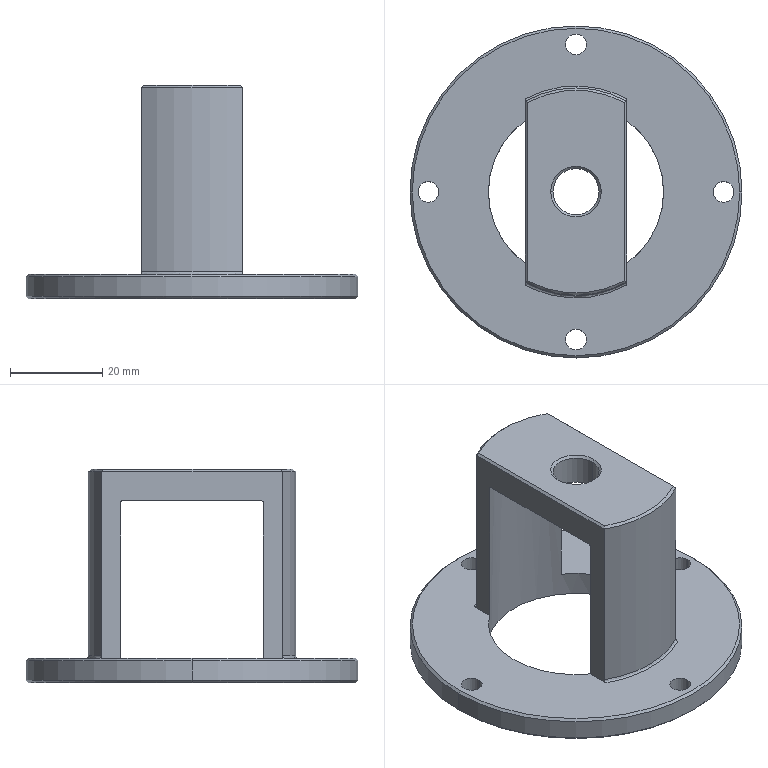Part | STEP file | Sensor mounting seat | 1 solid | 36 faces | box 72 x 72 x 46.3 mm | volume 26633 mm3 | cylinder 16 | cone 8 | plane 8 | spline 4 | commonest cylinder face diameters 4.5 x8 10 x2 38 x2 45 x2 72 x2